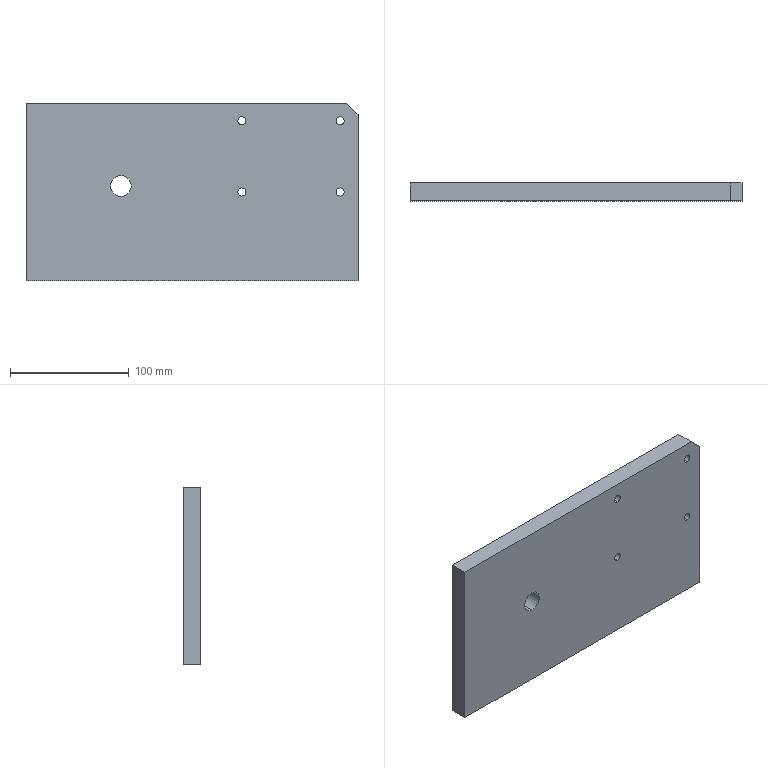Part | STEP file | A14-066 | 1 solid | 27 faces | box 280 x 15 x 150 mm | volume 623398 mm3 | cone 10 | cylinder 10 | plane 7 | commonest cylinder face diameters 6.8 x8 17.5 x2